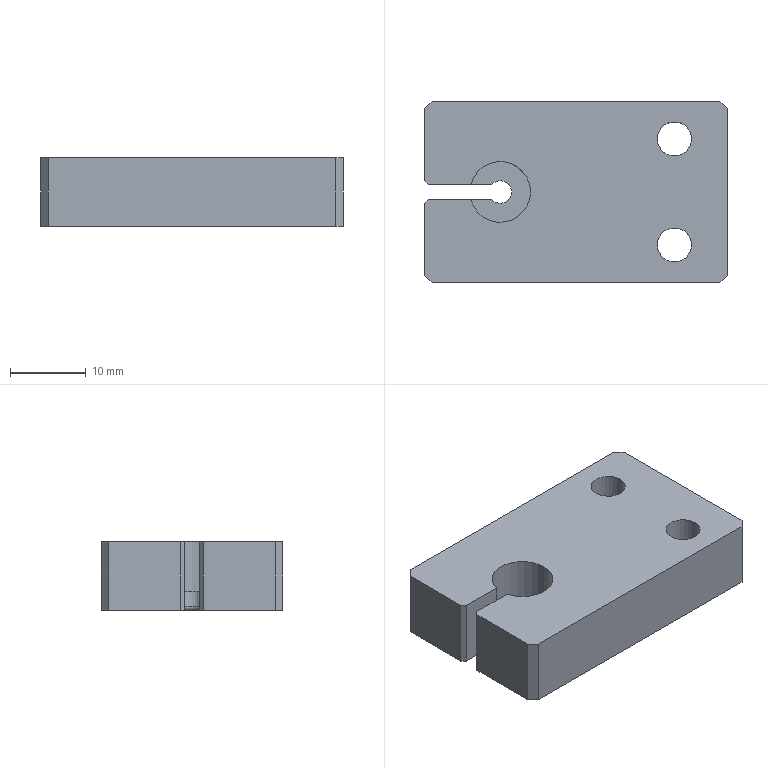Part | NX | 1 solid | 25 faces | box 40 x 24 x 9 mm | volume 7592 mm3 | plane 18 | cylinder 6 | torus 1 | commonest cylinder face diameters 8 x3 4.5 x2 3 x1
STEP:
#1=CARTESIAN_POINT('',(-20.,1.5,-9.));
#2=VERTEX_POINT('',#1);
#3=CARTESIAN_POINT('',(-19.5,1.,-9.));
#4=VERTEX_POINT('',#3);
#5=CARTESIAN_POINT('',(-19.75,1.25,-9.));
#6=DIRECTION('',(0.7071,-0.7071,0.));
#7=VECTOR('',#6,1000.);
#8=LINE('',#5,#7);
#9=EDGE_CURVE('',#2,#4,#8,.T.);
#10=ORIENTED_EDGE('',*,*,#9,.T.);
#11=CARTESIAN_POINT('',(-19.5,1.,0.));
#12=VERTEX_POINT('',#11);
#13=CARTESIAN_POINT('',(-19.5,1.,-4.5));
#14=DIRECTION('',(0.,0.,-1.));
#15=VECTOR('',#14,1000.);
#16=LINE('',#13,#15);
#17=EDGE_CURVE('',#12,#4,#16,.T.);
#18=ORIENTED_EDGE('',*,*,#17,.F.);
#19=CARTESIAN_POINT('',(-20.,1.5,0.));
#20=VERTEX_POINT('',#19);
#21=CARTESIAN_POINT('',(-19.75,1.25,0.));
#22=DIRECTION('',(0.7071,-0.7071,0.));
#23=VECTOR('',#22,1000.);
#24=LINE('',#21,#23);
#25=EDGE_CURVE('',#20,#12,#24,.T.);
#26=ORIENTED_EDGE('',*,*,#25,.F.);
#27=CARTESIAN_POINT('',(-20.,1.5,-4.5));
#28=DIRECTION('',(0.,0.,-1.));
#29=VECTOR('',#28,1000.);
#30=LINE('',#27,#29);
#31=EDGE_CURVE('',#20,#2,#30,.T.);
#32=ORIENTED_EDGE('',*,*,#31,.T.);
#33=EDGE_LOOP('',(#10,#18,#26,#32));
#34=FACE_BOUND('',#33,.T.);
#35=CARTESIAN_POINT('',(-20.,1.5,-4.5));
#36=DIRECTION('',(-0.7071,-0.7071,0.));
#37=DIRECTION('',(0.,0.,-1.));
#38=AXIS2_PLACEMENT_3D('',#35,#36,#37);
#39=PLANE('',#38);
#40=ADVANCED_FACE('',(#34),#39,.T.);
#41=CARTESIAN_POINT('',(9.,-7.,-9.));
#42=VERTEX_POINT('',#41);
#43=CARTESIAN_POINT('',(13.,-7.,-9.));
#44=DIRECTION('',(0.,0.,1.));
#45=DIRECTION('',(-1.,0.,0.));
#46=AXIS2_PLACEMENT_3D('',#43,#44,#45);
#47=CIRCLE('',#46,4.);
#48=EDGE_CURVE('',#42,#42,#47,.T.);
#49=ORIENTED_EDGE('',*,*,#48,.T.);
#50=EDGE_LOOP('',(#49));
#51=FACE_BOUND('',#50,.T.);
#52=CARTESIAN_POINT('',(17.,7.,-9.));
#53=VERTEX_POINT('',#52);
#54=CARTESIAN_POINT('',(13.,7.,-9.));
#55=DIRECTION('',(0.,0.,-1.));
#56=DIRECTION('',(1.,0.,0.));
#57=AXIS2_PLACEMENT_3D('',#54,#55,#56);
#58=CIRCLE('',#57,4.);
#59=EDGE_CURVE('',#53,#53,#58,.T.);
#60=ORIENTED_EDGE('',*,*,#59,.F.);
#61=EDGE_LOOP('',(#60));
#62=FACE_BOUND('',#61,.T.);
#63=CARTESIAN_POINT('',(-11.732,1.,-9.));
#64=VERTEX_POINT('',#63);
#65=CARTESIAN_POINT('',(-15.616,1.,-9.));
#66=DIRECTION('',(1.,0.,0.));
#67=VECTOR('',#66,1000.);
#68=LINE('',#65,#67);
#69=EDGE_CURVE('',#4,#64,#68,.T.);
#70=ORIENTED_EDGE('',*,*,#69,.F.);
#71=ORIENTED_EDGE('',*,*,#9,.F.);
#72=CARTESIAN_POINT('',(-20.,11.,-9.));
#73=VERTEX_POINT('',#72);
#74=CARTESIAN_POINT('',(-20.,6.25,-9.));
#75=DIRECTION('',(0.,-1.,0.));
#76=VECTOR('',#75,1000.);
#77=LINE('',#74,#76);
#78=EDGE_CURVE('',#73,#2,#77,.T.);
#79=ORIENTED_EDGE('',*,*,#78,.F.);
#80=CARTESIAN_POINT('',(-19.,12.,-9.));
#81=VERTEX_POINT('',#80);
#82=CARTESIAN_POINT('',(-19.5,11.5,-9.));
#83=DIRECTION('',(-0.7071,-0.7071,0.));
#84=VECTOR('',#83,1000.);
#85=LINE('',#82,#84);
#86=EDGE_CURVE('',#81,#73,#85,.T.);
#87=ORIENTED_EDGE('',*,*,#86,.F.);
#88=CARTESIAN_POINT('',(19.,12.,-9.));
#89=VERTEX_POINT('',#88);
#90=CARTESIAN_POINT('',(0.,12.,-9.));
#91=DIRECTION('',(-1.,0.,0.));
#92=VECTOR('',#91,1000.);
#93=LINE('',#90,#92);
#94=EDGE_CURVE('',#89,#81,#93,.T.);
#95=ORIENTED_EDGE('',*,*,#94,.F.);
#96=CARTESIAN_POINT('',(20.,11.,-9.));
#97=VERTEX_POINT('',#96);
#98=CARTESIAN_POINT('',(19.5,11.5,-9.));
#99=DIRECTION('',(-0.7071,0.7071,0.));
#100=VECTOR('',#99,1000.);
#101=LINE('',#98,#100);
#102=EDGE_CURVE('',#97,#89,#101,.T.);
#103=ORIENTED_EDGE('',*,*,#102,.F.);
#104=CARTESIAN_POINT('',(20.,-11.,-9.));
#105=VERTEX_POINT('',#104);
#106=CARTESIAN_POINT('',(20.,0.,-9.));
#107=DIRECTION('',(0.,1.,0.));
#108=VECTOR('',#107,1000.);
#109=LINE('',#106,#108);
#110=EDGE_CURVE('',#105,#97,#109,.T.);
#111=ORIENTED_EDGE('',*,*,#110,.F.);
#112=CARTESIAN_POINT('',(19.,-12.,-9.));
#113=VERTEX_POINT('',#112);
#114=CARTESIAN_POINT('',(19.5,-11.5,-9.));
#115=DIRECTION('',(0.7071,0.7071,0.));
#116=VECTOR('',#115,1000.);
#117=LINE('',#114,#116);
#118=EDGE_CURVE('',#113,#105,#117,.T.);
#119=ORIENTED_EDGE('',*,*,#118,.F.);
#120=CARTESIAN_POINT('',(-19.,-12.,-9.));
#121=VERTEX_POINT('',#120);
#122=CARTESIAN_POINT('',(0.,-12.,-9.));
#123=DIRECTION('',(1.,0.,0.));
#124=VECTOR('',#123,1000.);
#125=LINE('',#122,#124);
#126=EDGE_CURVE('',#121,#113,#125,.T.);
#127=ORIENTED_EDGE('',*,*,#126,.F.);
#128=CARTESIAN_POINT('',(-20.,-11.,-9.));
#129=VERTEX_POINT('',#128);
#130=CARTESIAN_POINT('',(-19.5,-11.5,-9.));
#131=DIRECTION('',(0.7071,-0.7071,0.));
#132=VECTOR('',#131,1000.);
#133=LINE('',#130,#132);
#134=EDGE_CURVE('',#129,#121,#133,.T.);
#135=ORIENTED_EDGE('',*,*,#134,.F.);
#136=CARTESIAN_POINT('',(-20.,-1.5,-9.));
#137=VERTEX_POINT('',#136);
#138=CARTESIAN_POINT('',(-20.,-6.25,-9.));
#139=DIRECTION('',(0.,-1.,0.));
#140=VECTOR('',#139,1000.);
#141=LINE('',#138,#140);
#142=EDGE_CURVE('',#137,#129,#141,.T.);
#143=ORIENTED_EDGE('',*,*,#142,.F.);
#144=CARTESIAN_POINT('',(-19.5,-1.,-9.));
#145=VERTEX_POINT('',#144);
#146=CARTESIAN_POINT('',(-19.75,-1.25,-9.));
#147=DIRECTION('',(-0.7071,-0.7071,0.));
#148=VECTOR('',#147,1000.);
#149=LINE('',#146,#148);
#150=EDGE_CURVE('',#145,#137,#149,.T.);
#151=ORIENTED_EDGE('',*,*,#150,.F.);
#152=CARTESIAN_POINT('',(-11.732,-1.,-9.));
#153=VERTEX_POINT('',#152);
#154=CARTESIAN_POINT('',(-15.616,-1.,-9.));
#155=DIRECTION('',(1.,0.,0.));
#156=VECTOR('',#155,1000.);
#157=LINE('',#154,#156);
#158=EDGE_CURVE('',#145,#153,#157,.T.);
#159=ORIENTED_EDGE('',*,*,#158,.T.);
#160=CARTESIAN_POINT('',(-10.,0.,-9.));
#161=DIRECTION('',(0.,0.,-1.));
#162=DIRECTION('',(1.,0.,0.));
#163=AXIS2_PLACEMENT_3D('',#160,#161,#162);
#164=CIRCLE('',#163,2.);
#165=EDGE_CURVE('',#64,#153,#164,.T.);
#166=ORIENTED_EDGE('',*,*,#165,.F.);
#167=EDGE_LOOP('',(#70,#71,#79,#87,#95,#103,#111,#119,#127,#135,#143,#151,#159,#166));
#168=FACE_BOUND('',#167,.T.);
#169=CARTESIAN_POINT('',(0.,0.,-9.));
#170=DIRECTION('',(0.,0.,-1.));
#171=DIRECTION('',(1.,0.,0.));
#172=AXIS2_PLACEMENT_3D('',#169,#170,#171);
#173=PLANE('',#172);
#174=ADVANCED_FACE('',(#51,#62,#168),#173,.T.);
#175=CARTESIAN_POINT('',(10.75,-7.,0.));
#176=VERTEX_POINT('',#175);
#177=CARTESIAN_POINT('',(13.,-7.,0.));
#178=DIRECTION('',(0.,0.,1.));
#179=DIRECTION('',(-1.,0.,0.));
#180=AXIS2_PLACEMENT_3D('',#177,#178,#179);
#181=CIRCLE('',#180,2.25);
#182=EDGE_CURVE('',#176,#176,#181,.T.);
#183=ORIENTED_EDGE('',*,*,#182,.F.);
#184=EDGE_LOOP('',(#183));
#185=FACE_BOUND('',#184,.T.);
#186=CARTESIAN_POINT('',(15.25,7.,0.));
#187=VERTEX_POINT('',#186);
#188=CARTESIAN_POINT('',(13.,7.,0.));
#189=DIRECTION('',(0.,0.,-1.));
#190=DIRECTION('',(1.,0.,0.));
#191=AXIS2_PLACEMENT_3D('',#188,#189,#190);
#192=CIRCLE('',#191,2.25);
#193=EDGE_CURVE('',#187,#187,#192,.T.);
#194=ORIENTED_EDGE('',*,*,#193,.T.);
#195=EDGE_LOOP('',(#194));
#196=FACE_BOUND('',#195,.T.);
#197=ORIENTED_EDGE('',*,*,#25,.T.);
#198=CARTESIAN_POINT('',(-13.873,1.,0.));
#199=VERTEX_POINT('',#198);
#200=CARTESIAN_POINT('',(-16.686,1.,0.));
#201=DIRECTION('',(1.,0.,0.));
#202=VECTOR('',#201,1000.);
#203=LINE('',#200,#202);
#204=EDGE_CURVE('',#12,#199,#203,.T.);
#205=ORIENTED_EDGE('',*,*,#204,.T.);
#206=CARTESIAN_POINT('',(-13.873,-1.,0.));
#207=VERTEX_POINT('',#206);
#208=CARTESIAN_POINT('',(-10.,0.,0.));
#209=DIRECTION('',(0.,0.,-1.));
#210=DIRECTION('',(1.,0.,0.));
#211=AXIS2_PLACEMENT_3D('',#208,#209,#210);
#212=CIRCLE('',#211,4.);
#213=EDGE_CURVE('',#199,#207,#212,.T.);
#214=ORIENTED_EDGE('',*,*,#213,.T.);
#215=CARTESIAN_POINT('',(-19.5,-1.,0.));
#216=VERTEX_POINT('',#215);
#217=CARTESIAN_POINT('',(-16.686,-1.,0.));
#218=DIRECTION('',(-1.,0.,0.));
#219=VECTOR('',#218,1000.);
#220=LINE('',#217,#219);
#221=EDGE_CURVE('',#207,#216,#220,.T.);
#222=ORIENTED_EDGE('',*,*,#221,.T.);
#223=CARTESIAN_POINT('',(-20.,-1.5,0.));
#224=VERTEX_POINT('',#223);
#225=CARTESIAN_POINT('',(-19.75,-1.25,0.));
#226=DIRECTION('',(-0.7071,-0.7071,0.));
#227=VECTOR('',#226,1000.);
#228=LINE('',#225,#227);
#229=EDGE_CURVE('',#216,#224,#228,.T.);
#230=ORIENTED_EDGE('',*,*,#229,.T.);
#231=CARTESIAN_POINT('',(-20.,-11.,0.));
#232=VERTEX_POINT('',#231);
#233=CARTESIAN_POINT('',(-20.,-6.25,0.));
#234=DIRECTION('',(0.,-1.,0.));
#235=VECTOR('',#234,1000.);
#236=LINE('',#233,#235);
#237=EDGE_CURVE('',#224,#232,#236,.T.);
#238=ORIENTED_EDGE('',*,*,#237,.T.);
#239=CARTESIAN_POINT('',(-19.,-12.,0.));
#240=VERTEX_POINT('',#239);
#241=CARTESIAN_POINT('',(-19.5,-11.5,0.));
#242=DIRECTION('',(0.7071,-0.7071,0.));
#243=VECTOR('',#242,1000.);
#244=LINE('',#241,#243);
#245=EDGE_CURVE('',#232,#240,#244,.T.);
#246=ORIENTED_EDGE('',*,*,#245,.T.);
#247=CARTESIAN_POINT('',(19.,-12.,0.));
#248=VERTEX_POINT('',#247);
#249=CARTESIAN_POINT('',(0.,-12.,0.));
#250=DIRECTION('',(1.,0.,0.));
#251=VECTOR('',#250,1000.);
#252=LINE('',#249,#251);
#253=EDGE_CURVE('',#240,#248,#252,.T.);
#254=ORIENTED_EDGE('',*,*,#253,.T.);
#255=CARTESIAN_POINT('',(20.,-11.,0.));
#256=VERTEX_POINT('',#255);
#257=CARTESIAN_POINT('',(19.5,-11.5,0.));
#258=DIRECTION('',(0.7071,0.7071,0.));
#259=VECTOR('',#258,1000.);
#260=LINE('',#257,#259);
#261=EDGE_CURVE('',#248,#256,#260,.T.);
#262=ORIENTED_EDGE('',*,*,#261,.T.);
#263=CARTESIAN_POINT('',(20.,11.,0.));
#264=VERTEX_POINT('',#263);
#265=CARTESIAN_POINT('',(20.,0.,0.));
#266=DIRECTION('',(0.,1.,0.));
#267=VECTOR('',#266,1000.);
#268=LINE('',#265,#267);
#269=EDGE_CURVE('',#256,#264,#268,.T.);
#270=ORIENTED_EDGE('',*,*,#269,.T.);
#271=CARTESIAN_POINT('',(19.,12.,0.));
#272=VERTEX_POINT('',#271);
#273=CARTESIAN_POINT('',(19.5,11.5,0.));
#274=DIRECTION('',(-0.7071,0.7071,0.));
#275=VECTOR('',#274,1000.);
#276=LINE('',#273,#275);
#277=EDGE_CURVE('',#264,#272,#276,.T.);
#278=ORIENTED_EDGE('',*,*,#277,.T.);
#279=CARTESIAN_POINT('',(-19.,12.,0.));
#280=VERTEX_POINT('',#279);
#281=CARTESIAN_POINT('',(0.,12.,0.));
#282=DIRECTION('',(-1.,0.,0.));
#283=VECTOR('',#282,1000.);
#284=LINE('',#281,#283);
#285=EDGE_CURVE('',#272,#280,#284,.T.);
#286=ORIENTED_EDGE('',*,*,#285,.T.);
#287=CARTESIAN_POINT('',(-20.,11.,0.));
#288=VERTEX_POINT('',#287);
#289=CARTESIAN_POINT('',(-19.5,11.5,0.));
#290=DIRECTION('',(-0.7071,-0.7071,0.));
#291=VECTOR('',#290,1000.);
#292=LINE('',#289,#291);
#293=EDGE_CURVE('',#280,#288,#292,.T.);
#294=ORIENTED_EDGE('',*,*,#293,.T.);
#295=CARTESIAN_POINT('',(-20.,6.25,0.));
#296=DIRECTION('',(0.,-1.,0.));
#297=VECTOR('',#296,1000.);
#298=LINE('',#295,#297);
#299=EDGE_CURVE('',#288,#20,#298,.T.);
#300=ORIENTED_EDGE('',*,*,#299,.T.);
#301=EDGE_LOOP('',(#197,#205,#214,#222,#230,#238,#246,#254,#262,#270,#278,#286,#294,#300));
#302=FACE_BOUND('',#301,.T.);
#303=CARTESIAN_POINT('',(0.,0.,0.));
#304=DIRECTION('',(0.,0.,-1.));
#305=DIRECTION('',(1.,0.,0.));
#306=AXIS2_PLACEMENT_3D('',#303,#304,#305);
#307=PLANE('',#306);
#308=ADVANCED_FACE('',(#185,#196,#302),#307,.F.);
#309=ORIENTED_EDGE('',*,*,#31,.F.);
#310=ORIENTED_EDGE('',*,*,#299,.F.);
#311=CARTESIAN_POINT('',(-20.,11.,-4.5));
#312=DIRECTION('',(0.,0.,-1.));
#313=VECTOR('',#312,1000.);
#314=LINE('',#311,#313);
#315=EDGE_CURVE('',#288,#73,#314,.T.);
#316=ORIENTED_EDGE('',*,*,#315,.T.);
#317=ORIENTED_EDGE('',*,*,#78,.T.);
#318=EDGE_LOOP('',(#309,#310,#316,#317));
#319=FACE_BOUND('',#318,.T.);
#320=CARTESIAN_POINT('',(-20.,12.,-4.5));
#321=DIRECTION('',(1.,0.,0.));
#322=DIRECTION('',(0.,-1.,0.));
#323=AXIS2_PLACEMENT_3D('',#320,#321,#322);
#324=PLANE('',#323);
#325=ADVANCED_FACE('',(#319),#324,.F.);
#326=CARTESIAN_POINT('',(-11.118,1.,-8.5));
#327=VERTEX_POINT('',#326);
#328=CARTESIAN_POINT('',(-11.118,1.,-8.5));
#329=CARTESIAN_POINT('',(-11.118,1.,-8.794));
#330=CARTESIAN_POINT('',(-11.439,1.,-9.));
#331=CARTESIAN_POINT('',(-11.732,1.,-9.));
#332=B_SPLINE_CURVE_WITH_KNOTS('',3,(#328,#329,#330,#331),.UNSPECIFIED.,.F.,.F.,(4,4),(0.,0.0008677),.UNSPECIFIED.);
#333=EDGE_CURVE('',#327,#64,#332,.T.);
#334=ORIENTED_EDGE('',*,*,#333,.F.);
#335=CARTESIAN_POINT('',(-11.118,1.,-6.5));
#336=VERTEX_POINT('',#335);
#337=CARTESIAN_POINT('',(-11.118,1.,-7.905));
#338=DIRECTION('',(0.,0.,-1.));
#339=VECTOR('',#338,1000.);
#340=LINE('',#337,#339);
#341=EDGE_CURVE('',#336,#327,#340,.T.);
#342=ORIENTED_EDGE('',*,*,#341,.F.);
#343=CARTESIAN_POINT('',(-13.873,1.,-6.5));
#344=VERTEX_POINT('',#343);
#345=CARTESIAN_POINT('',(-12.496,1.,-6.5));
#346=DIRECTION('',(-1.,0.,0.));
#347=VECTOR('',#346,1000.);
#348=LINE('',#345,#347);
#349=EDGE_CURVE('',#336,#344,#348,.T.);
#350=ORIENTED_EDGE('',*,*,#349,.T.);
#351=CARTESIAN_POINT('',(-13.873,1.,-3.095));
#352=DIRECTION('',(0.,0.,-1.));
#353=VECTOR('',#352,1000.);
#354=LINE('',#351,#353);
#355=EDGE_CURVE('',#199,#344,#354,.T.);
#356=ORIENTED_EDGE('',*,*,#355,.F.);
#357=ORIENTED_EDGE('',*,*,#204,.F.);
#358=ORIENTED_EDGE('',*,*,#17,.T.);
#359=ORIENTED_EDGE('',*,*,#69,.T.);
#360=EDGE_LOOP('',(#334,#342,#350,#356,#357,#358,#359));
#361=FACE_BOUND('',#360,.T.);
#362=CARTESIAN_POINT('',(-20.,1.,0.));
#363=DIRECTION('',(0.,1.,0.));
#364=DIRECTION('',(1.,0.,0.));
#365=AXIS2_PLACEMENT_3D('',#362,#363,#364);
#366=PLANE('',#365);
#367=ADVANCED_FACE('',(#361),#366,.F.);
#368=ORIENTED_EDGE('',*,*,#150,.T.);
#369=CARTESIAN_POINT('',(-20.,-1.5,-4.5));
#370=DIRECTION('',(0.,0.,-1.));
#371=VECTOR('',#370,1000.);
#372=LINE('',#369,#371);
#373=EDGE_CURVE('',#224,#137,#372,.T.);
#374=ORIENTED_EDGE('',*,*,#373,.F.);
#375=ORIENTED_EDGE('',*,*,#229,.F.);
#376=CARTESIAN_POINT('',(-19.5,-1.,-4.5));
#377=DIRECTION('',(0.,0.,-1.));
#378=VECTOR('',#377,1000.);
#379=LINE('',#376,#378);
#380=EDGE_CURVE('',#216,#145,#379,.T.);
#381=ORIENTED_EDGE('',*,*,#380,.T.);
#382=EDGE_LOOP('',(#368,#374,#375,#381));
#383=FACE_BOUND('',#382,.T.);
#384=CARTESIAN_POINT('',(-19.5,-1.,-4.5));
#385=DIRECTION('',(-0.7071,0.7071,0.));
#386=DIRECTION('',(0.,0.,-1.));
#387=AXIS2_PLACEMENT_3D('',#384,#385,#386);
#388=PLANE('',#387);
#389=ADVANCED_FACE('',(#383),#388,.T.);
#390=ORIENTED_EDGE('',*,*,#373,.T.);
#391=ORIENTED_EDGE('',*,*,#142,.T.);
#392=CARTESIAN_POINT('',(-20.,-11.,-4.5));
#393=DIRECTION('',(0.,0.,-1.));
#394=VECTOR('',#393,1000.);
#395=LINE('',#392,#394);
#396=EDGE_CURVE('',#232,#129,#395,.T.);
#397=ORIENTED_EDGE('',*,*,#396,.F.);
#398=ORIENTED_EDGE('',*,*,#237,.F.);
#399=EDGE_LOOP('',(#390,#391,#397,#398));
#400=FACE_BOUND('',#399,.T.);
#401=CARTESIAN_POINT('',(-20.,12.,-4.5));
#402=DIRECTION('',(1.,0.,0.));
#403=DIRECTION('',(0.,-1.,0.));
#404=AXIS2_PLACEMENT_3D('',#401,#402,#403);
#405=PLANE('',#404);
#406=ADVANCED_FACE('',(#400),#405,.F.);
#407=CARTESIAN_POINT('',(-11.118,-1.,-8.5));
#408=VERTEX_POINT('',#407);
#409=CARTESIAN_POINT('',(-11.118,-1.,-8.5));
#410=CARTESIAN_POINT('',(-11.118,-1.,-8.794));
#411=CARTESIAN_POINT('',(-11.439,-1.,-9.));
#412=CARTESIAN_POINT('',(-11.732,-1.,-9.));
#413=B_SPLINE_CURVE_WITH_KNOTS('',3,(#409,#410,#411,#412),.UNSPECIFIED.,.F.,.F.,(4,4),(0.,0.0008677),.UNSPECIFIED.);
#414=EDGE_CURVE('',#408,#153,#413,.T.);
#415=ORIENTED_EDGE('',*,*,#414,.T.);
#416=ORIENTED_EDGE('',*,*,#158,.F.);
#417=ORIENTED_EDGE('',*,*,#380,.F.);
#418=ORIENTED_EDGE('',*,*,#221,.F.);
#419=CARTESIAN_POINT('',(-13.873,-1.,-6.5));
#420=VERTEX_POINT('',#419);
#421=CARTESIAN_POINT('',(-13.873,-1.,-3.095));
#422=DIRECTION('',(0.,0.,-1.));
#423=VECTOR('',#422,1000.);
#424=LINE('',#421,#423);
#425=EDGE_CURVE('',#207,#420,#424,.T.);
#426=ORIENTED_EDGE('',*,*,#425,.T.);
#427=CARTESIAN_POINT('',(-11.118,-1.,-6.5));
#428=VERTEX_POINT('',#427);
#429=CARTESIAN_POINT('',(-12.496,-1.,-6.5));
#430=DIRECTION('',(-1.,0.,0.));
#431=VECTOR('',#430,1000.);
#432=LINE('',#429,#431);
#433=EDGE_CURVE('',#428,#420,#432,.T.);
#434=ORIENTED_EDGE('',*,*,#433,.F.);
#435=CARTESIAN_POINT('',(-11.118,-1.,-7.905));
#436=DIRECTION('',(0.,0.,-1.));
#437=VECTOR('',#436,1000.);
#438=LINE('',#435,#437);
#439=EDGE_CURVE('',#428,#408,#438,.T.);
#440=ORIENTED_EDGE('',*,*,#439,.T.);
#441=EDGE_LOOP('',(#415,#416,#417,#418,#426,#434,#440));
#442=FACE_BOUND('',#441,.T.);
#443=CARTESIAN_POINT('',(-10.,-1.,0.));
#444=DIRECTION('',(0.,-1.,0.));
#445=DIRECTION('',(-1.,0.,0.));
#446=AXIS2_PLACEMENT_3D('',#443,#444,#445);
#447=PLANE('',#446);
#448=ADVANCED_FACE('',(#442),#447,.F.);
#449=ORIENTED_EDGE('',*,*,#86,.T.);
#450=ORIENTED_EDGE('',*,*,#315,.F.);
#451=ORIENTED_EDGE('',*,*,#293,.F.);
#452=CARTESIAN_POINT('',(-19.,12.,-4.5));
#453=DIRECTION('',(0.,0.,-1.));
#454=VECTOR('',#453,1000.);
#455=LINE('',#452,#454);
#456=EDGE_CURVE('',#280,#81,#455,.T.);
#457=ORIENTED_EDGE('',*,*,#456,.T.);
#458=EDGE_LOOP('',(#449,#450,#451,#457));
#459=FACE_BOUND('',#458,.T.);
#460=CARTESIAN_POINT('',(-19.,12.,-4.5));
#461=DIRECTION('',(-0.7071,0.7071,0.));
#462=DIRECTION('',(0.,0.,-1.));
#463=AXIS2_PLACEMENT_3D('',#460,#461,#462);
#464=PLANE('',#463);
#465=ADVANCED_FACE('',(#459),#464,.T.);
#466=ORIENTED_EDGE('',*,*,#456,.F.);
#467=ORIENTED_EDGE('',*,*,#285,.F.);
#468=CARTESIAN_POINT('',(19.,12.,-4.5));
#469=DIRECTION('',(0.,0.,-1.));
#470=VECTOR('',#469,1000.);
#471=LINE('',#468,#470);
#472=EDGE_CURVE('',#272,#89,#471,.T.);
#473=ORIENTED_EDGE('',*,*,#472,.T.);
#474=ORIENTED_EDGE('',*,*,#94,.T.);
#475=EDGE_LOOP('',(#466,#467,#473,#474));
#476=FACE_BOUND('',#475,.T.);
#477=CARTESIAN_POINT('',(20.,12.,-4.5));
#478=DIRECTION('',(0.,-1.,0.));
#479=DIRECTION('',(-1.,0.,0.));
#480=AXIS2_PLACEMENT_3D('',#477,#478,#479);
#481=PLANE('',#480);
#482=ADVANCED_FACE('',(#476),#481,.F.);
#483=ORIENTED_EDGE('',*,*,#102,.T.);
#484=ORIENTED_EDGE('',*,*,#472,.F.);
#485=ORIENTED_EDGE('',*,*,#277,.F.);
#486=CARTESIAN_POINT('',(20.,11.,-4.5));
#487=DIRECTION('',(0.,0.,-1.));
#488=VECTOR('',#487,1000.);
#489=LINE('',#486,#488);
#490=EDGE_CURVE('',#264,#97,#489,.T.);
#491=ORIENTED_EDGE('',*,*,#490,.T.);
#492=EDGE_LOOP('',(#483,#484,#485,#491));
#493=FACE_BOUND('',#492,.T.);
#494=CARTESIAN_POINT('',(20.,11.,-4.5));
#495=DIRECTION('',(0.7071,0.7071,0.));
#496=DIRECTION('',(0.,0.,-1.));
#497=AXIS2_PLACEMENT_3D('',#494,#495,#496);
#498=PLANE('',#497);
#499=ADVANCED_FACE('',(#493),#498,.T.);
#500=ORIENTED_EDGE('',*,*,#490,.F.);
#501=ORIENTED_EDGE('',*,*,#269,.F.);
#502=CARTESIAN_POINT('',(20.,-11.,-4.5));
#503=DIRECTION('',(0.,0.,-1.));
#504=VECTOR('',#503,1000.);
#505=LINE('',#502,#504);
#506=EDGE_CURVE('',#256,#105,#505,.T.);
#507=ORIENTED_EDGE('',*,*,#506,.T.);
#508=ORIENTED_EDGE('',*,*,#110,.T.);
#509=EDGE_LOOP('',(#500,#501,#507,#508));
#510=FACE_BOUND('',#509,.T.);
#511=CARTESIAN_POINT('',(20.,-12.,-4.5));
#512=DIRECTION('',(-1.,0.,0.));
#513=DIRECTION('',(0.,1.,0.));
#514=AXIS2_PLACEMENT_3D('',#511,#512,#513);
#515=PLANE('',#514);
#516=ADVANCED_FACE('',(#510),#515,.F.);
#517=ORIENTED_EDGE('',*,*,#118,.T.);
#518=ORIENTED_EDGE('',*,*,#506,.F.);
#519=ORIENTED_EDGE('',*,*,#261,.F.);
#520=CARTESIAN_POINT('',(19.,-12.,-4.5));
#521=DIRECTION('',(0.,0.,-1.));
#522=VECTOR('',#521,1000.);
#523=LINE('',#520,#522);
#524=EDGE_CURVE('',#248,#113,#523,.T.);
#525=ORIENTED_EDGE('',*,*,#524,.T.);
#526=EDGE_LOOP('',(#517,#518,#519,#525));
#527=FACE_BOUND('',#526,.T.);
#528=CARTESIAN_POINT('',(19.,-12.,-4.5));
#529=DIRECTION('',(0.7071,-0.7071,0.));
#530=DIRECTION('',(0.,0.,-1.));
#531=AXIS2_PLACEMENT_3D('',#528,#529,#530);
#532=PLANE('',#531);
#533=ADVANCED_FACE('',(#527),#532,.T.);
#534=ORIENTED_EDGE('',*,*,#524,.F.);
#535=ORIENTED_EDGE('',*,*,#253,.F.);
#536=CARTESIAN_POINT('',(-19.,-12.,-4.5));
#537=DIRECTION('',(0.,0.,-1.));
#538=VECTOR('',#537,1000.);
#539=LINE('',#536,#538);
#540=EDGE_CURVE('',#240,#121,#539,.T.);
#541=ORIENTED_EDGE('',*,*,#540,.T.);
#542=ORIENTED_EDGE('',*,*,#126,.T.);
#543=EDGE_LOOP('',(#534,#535,#541,#542));
#544=FACE_BOUND('',#543,.T.);
#545=CARTESIAN_POINT('',(-20.,-12.,-4.5));
#546=DIRECTION('',(0.,1.,0.));
#547=DIRECTION('',(1.,0.,0.));
#548=AXIS2_PLACEMENT_3D('',#545,#546,#547);
#549=PLANE('',#548);
#550=ADVANCED_FACE('',(#544),#549,.F.);
#551=ORIENTED_EDGE('',*,*,#134,.T.);
#552=ORIENTED_EDGE('',*,*,#540,.F.);
#553=ORIENTED_EDGE('',*,*,#245,.F.);
#554=ORIENTED_EDGE('',*,*,#396,.T.);
#555=EDGE_LOOP('',(#551,#552,#553,#554));
#556=FACE_BOUND('',#555,.T.);
#557=CARTESIAN_POINT('',(-20.,-11.,-4.5));
#558=DIRECTION('',(-0.7071,-0.7071,0.));
#559=DIRECTION('',(0.,0.,-1.));
#560=AXIS2_PLACEMENT_3D('',#557,#558,#559);
#561=PLANE('',#560);
#562=ADVANCED_FACE('',(#556),#561,.T.);
#563=CARTESIAN_POINT('',(10.75,7.,-5.));
#564=VERTEX_POINT('',#563);
#565=CARTESIAN_POINT('',(13.,7.,-5.));
#566=DIRECTION('',(0.,0.,1.));
#567=DIRECTION('',(-1.,0.,0.));
#568=AXIS2_PLACEMENT_3D('',#565,#566,#567);
#569=CIRCLE('',#568,2.25);
#570=EDGE_CURVE('',#564,#564,#569,.T.);
#571=ORIENTED_EDGE('',*,*,#570,.F.);
#572=EDGE_LOOP('',(#571));
#573=FACE_BOUND('',#572,.T.);
#574=ORIENTED_EDGE('',*,*,#193,.F.);
#575=EDGE_LOOP('',(#574));
#576=FACE_BOUND('',#575,.T.);
#577=CARTESIAN_POINT('',(13.,7.,-9.));
#578=DIRECTION('',(0.,0.,-1.));
#579=DIRECTION('',(1.,0.,0.));
#580=AXIS2_PLACEMENT_3D('',#577,#578,#579);
#581=CYLINDRICAL_SURFACE('',#580,2.25);
#582=ADVANCED_FACE('',(#573,#576),#581,.F.);
#583=CARTESIAN_POINT('',(9.,-7.,-5.));
#584=VERTEX_POINT('',#583);
#585=CARTESIAN_POINT('',(13.,-7.,-5.));
#586=DIRECTION('',(0.,0.,1.));
#587=DIRECTION('',(-1.,0.,0.));
#588=AXIS2_PLACEMENT_3D('',#585,#586,#587);
#589=CIRCLE('',#588,4.);
#590=EDGE_CURVE('',#584,#584,#589,.T.);
#591=ORIENTED_EDGE('',*,*,#590,.T.);
#592=EDGE_LOOP('',(#591));
#593=FACE_BOUND('',#592,.T.);
#594=ORIENTED_EDGE('',*,*,#48,.F.);
#595=EDGE_LOOP('',(#594));
#596=FACE_BOUND('',#595,.T.);
#597=CARTESIAN_POINT('',(13.,-7.,-9.));
#598=DIRECTION('',(0.,0.,1.));
#599=DIRECTION('',(1.,0.,0.));
#600=AXIS2_PLACEMENT_3D('',#597,#598,#599);
#601=CYLINDRICAL_SURFACE('',#600,4.);
#602=ADVANCED_FACE('',(#593,#596),#601,.F.);
#603=CARTESIAN_POINT('',(10.75,-7.,-5.));
#604=VERTEX_POINT('',#603);
#605=CARTESIAN_POINT('',(13.,-7.,-5.));
#606=DIRECTION('',(0.,0.,1.));
#607=DIRECTION('',(-1.,0.,0.));
#608=AXIS2_PLACEMENT_3D('',#605,#606,#607);
#609=CIRCLE('',#608,2.25);
#610=EDGE_CURVE('',#604,#604,#609,.T.);
#611=ORIENTED_EDGE('',*,*,#610,.T.);
#612=EDGE_LOOP('',(#611));
#613=FACE_BOUND('',#612,.T.);
#614=ORIENTED_EDGE('',*,*,#590,.F.);
#615=EDGE_LOOP('',(#614));
#616=FACE_BOUND('',#615,.T.);
#617=CARTESIAN_POINT('',(15.25,-7.,-5.));
#618=DIRECTION('',(0.,0.,1.));
#619=DIRECTION('',(1.,0.,0.));
#620=AXIS2_PLACEMENT_3D('',#617,#618,#619);
#621=PLANE('',#620);
#622=ADVANCED_FACE('',(#613,#616),#621,.F.);
#623=ORIENTED_EDGE('',*,*,#570,.T.);
#624=EDGE_LOOP('',(#623));
#625=FACE_BOUND('',#624,.T.);
#626=CARTESIAN_POINT('',(17.,7.,-5.));
#627=VERTEX_POINT('',#626);
#628=CARTESIAN_POINT('',(13.,7.,-5.));
#629=DIRECTION('',(0.,0.,-1.));
#630=DIRECTION('',(1.,0.,0.));
#631=AXIS2_PLACEMENT_3D('',#628,#629,#630);
#632=CIRCLE('',#631,4.);
#633=EDGE_CURVE('',#627,#627,#632,.T.);
#634=ORIENTED_EDGE('',*,*,#633,.T.);
#635=EDGE_LOOP('',(#634));
#636=FACE_BOUND('',#635,.T.);
#637=CARTESIAN_POINT('',(15.25,-7.,-5.));
#638=DIRECTION('',(0.,0.,1.));
#639=DIRECTION('',(1.,0.,0.));
#640=AXIS2_PLACEMENT_3D('',#637,#638,#639);
#641=PLANE('',#640);
#642=ADVANCED_FACE('',(#625,#636),#641,.F.);
#643=ORIENTED_EDGE('',*,*,#59,.T.);
#644=EDGE_LOOP('',(#643));
#645=FACE_BOUND('',#644,.T.);
#646=ORIENTED_EDGE('',*,*,#633,.F.);
#647=EDGE_LOOP('',(#646));
#648=FACE_BOUND('',#647,.T.);
#649=CARTESIAN_POINT('',(13.,7.,-9.));
#650=DIRECTION('',(0.,0.,-1.));
#651=DIRECTION('',(1.,0.,0.));
#652=AXIS2_PLACEMENT_3D('',#649,#650,#651);
#653=CYLINDRICAL_SURFACE('',#652,4.);
#654=ADVANCED_FACE('',(#645,#648),#653,.F.);
#655=CARTESIAN_POINT('',(-10.,0.,-8.5));
#656=DIRECTION('',(0.,0.,-1.));
#657=DIRECTION('',(1.,0.,0.));
#658=AXIS2_PLACEMENT_3D('',#655,#656,#657);
#659=CIRCLE('',#658,1.5);
#660=EDGE_CURVE('',#327,#408,#659,.T.);
#661=ORIENTED_EDGE('',*,*,#660,.F.);
#662=ORIENTED_EDGE('',*,*,#333,.T.);
#663=ORIENTED_EDGE('',*,*,#165,.T.);
#664=ORIENTED_EDGE('',*,*,#414,.F.);
#665=EDGE_LOOP('',(#661,#662,#663,#664));
#666=FACE_BOUND('',#665,.T.);
#667=CARTESIAN_POINT('',(-10.,0.,-8.5));
#668=DIRECTION('',(0.,0.,-1.));
#669=DIRECTION('',(1.,0.,0.));
#670=AXIS2_PLACEMENT_3D('',#667,#668,#669);
#671=TOROIDAL_SURFACE('',#670,2.,0.5);
#672=ADVANCED_FACE('',(#666),#671,.T.);
#673=ORIENTED_EDGE('',*,*,#660,.T.);
#674=ORIENTED_EDGE('',*,*,#439,.F.);
#675=CARTESIAN_POINT('',(-10.,0.,-6.5));
#676=DIRECTION('',(0.,0.,-1.));
#677=DIRECTION('',(1.,0.,0.));
#678=AXIS2_PLACEMENT_3D('',#675,#676,#677);
#679=CIRCLE('',#678,1.5);
#680=EDGE_CURVE('',#336,#428,#679,.T.);
#681=ORIENTED_EDGE('',*,*,#680,.F.);
#682=ORIENTED_EDGE('',*,*,#341,.T.);
#683=EDGE_LOOP('',(#673,#674,#681,#682));
#684=FACE_BOUND('',#683,.T.);
#685=CARTESIAN_POINT('',(-10.,0.,0.));
#686=DIRECTION('',(0.,0.,-1.));
#687=DIRECTION('',(1.,0.,0.));
#688=AXIS2_PLACEMENT_3D('',#685,#686,#687);
#689=CYLINDRICAL_SURFACE('',#688,1.5);
#690=ADVANCED_FACE('',(#684),#689,.F.);
#691=ORIENTED_EDGE('',*,*,#182,.T.);
#692=EDGE_LOOP('',(#691));
#693=FACE_BOUND('',#692,.T.);
#694=ORIENTED_EDGE('',*,*,#610,.F.);
#695=EDGE_LOOP('',(#694));
#696=FACE_BOUND('',#695,.T.);
#697=CARTESIAN_POINT('',(13.,-7.,-9.));
#698=DIRECTION('',(0.,0.,1.));
#699=DIRECTION('',(1.,0.,0.));
#700=AXIS2_PLACEMENT_3D('',#697,#698,#699);
#701=CYLINDRICAL_SURFACE('',#700,2.25);
#702=ADVANCED_FACE('',(#693,#696),#701,.F.);
#703=ORIENTED_EDGE('',*,*,#213,.F.);
#704=ORIENTED_EDGE('',*,*,#355,.T.);
#705=CARTESIAN_POINT('',(-10.,0.,-6.5));
#706=DIRECTION('',(0.,0.,-1.));
#707=DIRECTION('',(1.,0.,0.));
#708=AXIS2_PLACEMENT_3D('',#705,#706,#707);
#709=CIRCLE('',#708,4.);
#710=EDGE_CURVE('',#344,#420,#709,.T.);
#711=ORIENTED_EDGE('',*,*,#710,.T.);
#712=ORIENTED_EDGE('',*,*,#425,.F.);
#713=EDGE_LOOP('',(#703,#704,#711,#712));
#714=FACE_BOUND('',#713,.T.);
#715=CARTESIAN_POINT('',(-10.,0.,0.));
#716=DIRECTION('',(0.,0.,-1.));
#717=DIRECTION('',(1.,0.,0.));
#718=AXIS2_PLACEMENT_3D('',#715,#716,#717);
#719=CYLINDRICAL_SURFACE('',#718,4.);
#720=ADVANCED_FACE('',(#714),#719,.F.);
#721=ORIENTED_EDGE('',*,*,#349,.F.);
#722=ORIENTED_EDGE('',*,*,#680,.T.);
#723=ORIENTED_EDGE('',*,*,#433,.T.);
#724=ORIENTED_EDGE('',*,*,#710,.F.);
#725=EDGE_LOOP('',(#721,#722,#723,#724));
#726=FACE_BOUND('',#725,.T.);
#727=CARTESIAN_POINT('',(-8.5,0.,-6.5));
#728=DIRECTION('',(0.,0.,-1.));
#729=DIRECTION('',(1.,0.,0.));
#730=AXIS2_PLACEMENT_3D('',#727,#728,#729);
#731=PLANE('',#730);
#732=ADVANCED_FACE('',(#726),#731,.F.);
#733=CLOSED_SHELL('',(#40,#174,#308,#325,#367,#389,#406,#448,#465,#482,#499,#516,#533,#550,#562,#582,#602,#622,#642,#654,#672,#690,#702,#720,#732));
#734=MANIFOLD_SOLID_BREP('',#733);
#735=(LENGTH_UNIT()NAMED_UNIT(*)SI_UNIT(.MILLI.,.METRE.));
#736=UNCERTAINTY_MEASURE_WITH_UNIT(LENGTH_MEASURE(0.0508),#735,'','');
#737=(NAMED_UNIT(*)PLANE_ANGLE_UNIT()SI_UNIT($,.RADIAN.));
#738=(NAMED_UNIT(*)SI_UNIT($,.STERADIAN.)SOLID_ANGLE_UNIT());
#739=(GEOMETRIC_REPRESENTATION_CONTEXT(3)GLOBAL_UNCERTAINTY_ASSIGNED_CONTEXT((#736))GLOBAL_UNIT_ASSIGNED_CONTEXT((#735,#737,#738))REPRESENTATION_CONTEXT('',''));
#740=ADVANCED_BREP_SHAPE_REPRESENTATION('',(#734),#739);